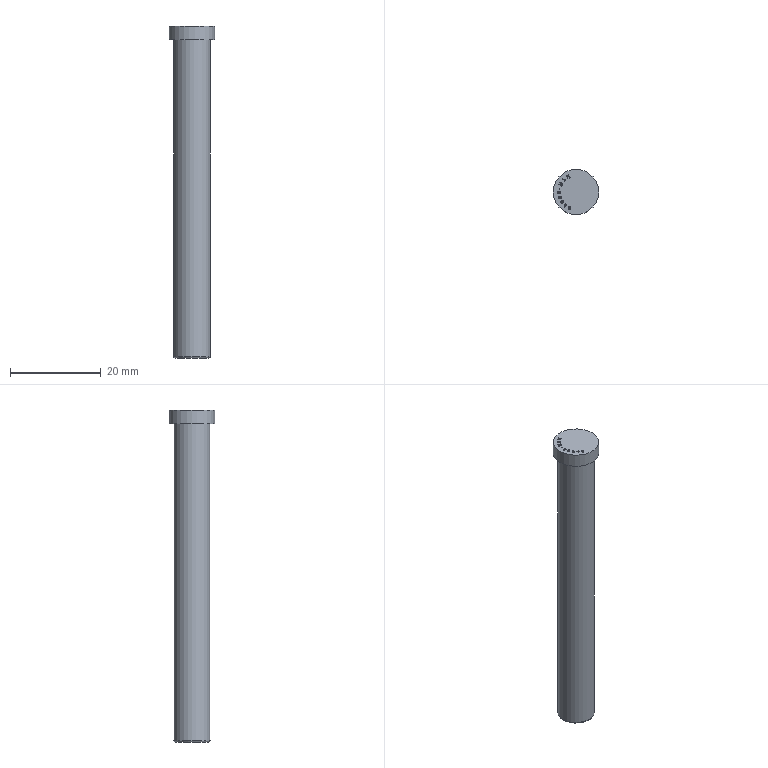Part | STEP file | lll_id2162_x_t | 1 solid | 89 faces | box 10 x 10 x 73 mm | volume 3753 mm3 | plane 61 | other 25 | cylinder 2 | torus 1 | commonest cylinder face diameters 8 x1 10 x1